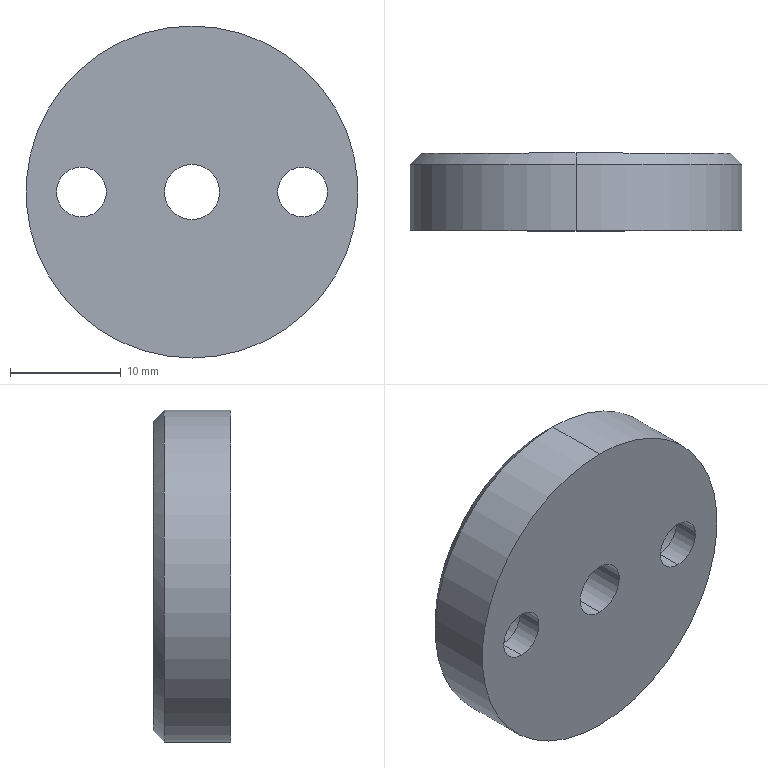Part | STEP file | 手柄盖^回墨刀-350 | 1 solid | 18 faces | box 30 x 7 x 30 mm | volume 4226 mm3 | cylinder 12 | plane 4 | cone 2 | commonest cylinder face diameters 4.5 x4 8 x4 5 x2 30 x2
STEP:
#1=CARTESIAN_POINT('',(-94.996,86.9,-6.23));
#2=VERTEX_POINT('',#1);
#3=CARTESIAN_POINT('',(-94.996,86.9,1.77));
#4=VERTEX_POINT('',#3);
#5=CARTESIAN_POINT('',(-94.996,86.9,-2.23));
#6=DIRECTION('',(0.,1.,0.));
#7=DIRECTION('',(0.,0.,1.));
#8=AXIS2_PLACEMENT_3D('',#5,#6,#7);
#9=CIRCLE('',#8,4.);
#10=EDGE_CURVE('',#2,#4,#9,.T.);
#11=ORIENTED_EDGE('',*,*,#10,.F.);
#12=CARTESIAN_POINT('',(-94.996,91.5,-6.23));
#13=VERTEX_POINT('',#12);
#14=CARTESIAN_POINT('',(-94.996,91.5,-6.23));
#15=DIRECTION('',(0.,1.,0.));
#16=VECTOR('',#15,1000.);
#17=LINE('',#14,#16);
#18=EDGE_CURVE('',#2,#13,#17,.T.);
#19=ORIENTED_EDGE('',*,*,#18,.T.);
#20=CARTESIAN_POINT('',(-94.996,91.5,1.77));
#21=VERTEX_POINT('',#20);
#22=CARTESIAN_POINT('',(-94.996,91.5,-2.23));
#23=DIRECTION('',(0.,1.,0.));
#24=DIRECTION('',(0.,0.,1.));
#25=AXIS2_PLACEMENT_3D('',#22,#23,#24);
#26=CIRCLE('',#25,4.);
#27=EDGE_CURVE('',#13,#21,#26,.T.);
#28=ORIENTED_EDGE('',*,*,#27,.T.);
#29=CARTESIAN_POINT('',(-94.996,91.5,1.77));
#30=DIRECTION('',(0.,1.,0.));
#31=VECTOR('',#30,1000.);
#32=LINE('',#29,#31);
#33=EDGE_CURVE('',#4,#21,#32,.T.);
#34=ORIENTED_EDGE('',*,*,#33,.F.);
#35=EDGE_LOOP('',(#11,#19,#28,#34));
#36=FACE_OUTER_BOUND('',#35,.T.);
#37=CARTESIAN_POINT('',(-94.996,91.5,-2.23));
#38=DIRECTION('',(0.,1.,0.));
#39=DIRECTION('',(0.,0.,1.));
#40=AXIS2_PLACEMENT_3D('',#37,#38,#39);
#41=CYLINDRICAL_SURFACE('',#40,4.);
#42=ADVANCED_FACE('',(#36),#41,.F.);
#43=CARTESIAN_POINT('',(-94.996,84.5,-4.48));
#44=VERTEX_POINT('',#43);
#45=CARTESIAN_POINT('',(-94.996,84.5,0.01978));
#46=VERTEX_POINT('',#45);
#47=CARTESIAN_POINT('',(-94.996,84.5,-2.23));
#48=DIRECTION('',(0.,1.,0.));
#49=DIRECTION('',(0.,0.,1.));
#50=AXIS2_PLACEMENT_3D('',#47,#48,#49);
#51=CIRCLE('',#50,2.25);
#52=EDGE_CURVE('',#44,#46,#51,.T.);
#53=ORIENTED_EDGE('',*,*,#52,.F.);
#54=CARTESIAN_POINT('',(-94.996,86.9,-4.48));
#55=VERTEX_POINT('',#54);
#56=CARTESIAN_POINT('',(-94.996,91.5,-4.48));
#57=DIRECTION('',(0.,1.,0.));
#58=VECTOR('',#57,1000.);
#59=LINE('',#56,#58);
#60=EDGE_CURVE('',#44,#55,#59,.T.);
#61=ORIENTED_EDGE('',*,*,#60,.T.);
#62=CARTESIAN_POINT('',(-94.996,86.9,0.01978));
#63=VERTEX_POINT('',#62);
#64=CARTESIAN_POINT('',(-94.996,86.9,-2.23));
#65=DIRECTION('',(0.,1.,0.));
#66=DIRECTION('',(0.,0.,1.));
#67=AXIS2_PLACEMENT_3D('',#64,#65,#66);
#68=CIRCLE('',#67,2.25);
#69=EDGE_CURVE('',#55,#63,#68,.T.);
#70=ORIENTED_EDGE('',*,*,#69,.T.);
#71=CARTESIAN_POINT('',(-94.996,91.5,0.01978));
#72=DIRECTION('',(0.,1.,0.));
#73=VECTOR('',#72,1000.);
#74=LINE('',#71,#73);
#75=EDGE_CURVE('',#46,#63,#74,.T.);
#76=ORIENTED_EDGE('',*,*,#75,.F.);
#77=EDGE_LOOP('',(#53,#61,#70,#76));
#78=FACE_OUTER_BOUND('',#77,.T.);
#79=CARTESIAN_POINT('',(-94.996,91.5,-2.23));
#80=DIRECTION('',(0.,1.,0.));
#81=DIRECTION('',(0.,0.,1.));
#82=AXIS2_PLACEMENT_3D('',#79,#80,#81);
#83=CYLINDRICAL_SURFACE('',#82,2.25);
#84=ADVANCED_FACE('',(#78),#83,.F.);
#85=CARTESIAN_POINT('',(-114.996,86.9,-6.23));
#86=VERTEX_POINT('',#85);
#87=CARTESIAN_POINT('',(-114.996,86.9,1.77));
#88=VERTEX_POINT('',#87);
#89=CARTESIAN_POINT('',(-114.996,86.9,-2.23));
#90=DIRECTION('',(0.,1.,0.));
#91=DIRECTION('',(0.,0.,1.));
#92=AXIS2_PLACEMENT_3D('',#89,#90,#91);
#93=CIRCLE('',#92,4.);
#94=EDGE_CURVE('',#86,#88,#93,.T.);
#95=ORIENTED_EDGE('',*,*,#94,.F.);
#96=CARTESIAN_POINT('',(-114.996,91.5,-6.23));
#97=VERTEX_POINT('',#96);
#98=CARTESIAN_POINT('',(-114.996,91.5,-6.23));
#99=DIRECTION('',(0.,1.,0.));
#100=VECTOR('',#99,1000.);
#101=LINE('',#98,#100);
#102=EDGE_CURVE('',#86,#97,#101,.T.);
#103=ORIENTED_EDGE('',*,*,#102,.T.);
#104=CARTESIAN_POINT('',(-118.996,91.5,-2.23));
#105=VERTEX_POINT('',#104);
#106=CARTESIAN_POINT('',(-114.996,91.5,-2.23));
#107=DIRECTION('',(0.,1.,0.));
#108=DIRECTION('',(0.,0.,1.));
#109=AXIS2_PLACEMENT_3D('',#106,#107,#108);
#110=CIRCLE('',#109,4.);
#111=EDGE_CURVE('',#97,#105,#110,.T.);
#112=ORIENTED_EDGE('',*,*,#111,.T.);
#113=CARTESIAN_POINT('',(-114.996,91.5,1.77));
#114=VERTEX_POINT('',#113);
#115=CARTESIAN_POINT('',(-114.996,91.5,-2.23));
#116=DIRECTION('',(0.,1.,0.));
#117=DIRECTION('',(0.,0.,1.));
#118=AXIS2_PLACEMENT_3D('',#115,#116,#117);
#119=CIRCLE('',#118,4.);
#120=EDGE_CURVE('',#105,#114,#119,.T.);
#121=ORIENTED_EDGE('',*,*,#120,.T.);
#122=CARTESIAN_POINT('',(-114.996,91.5,1.77));
#123=DIRECTION('',(0.,1.,0.));
#124=VECTOR('',#123,1000.);
#125=LINE('',#122,#124);
#126=EDGE_CURVE('',#88,#114,#125,.T.);
#127=ORIENTED_EDGE('',*,*,#126,.F.);
#128=EDGE_LOOP('',(#95,#103,#112,#121,#127));
#129=FACE_OUTER_BOUND('',#128,.T.);
#130=CARTESIAN_POINT('',(-114.996,91.5,-2.23));
#131=DIRECTION('',(0.,1.,0.));
#132=DIRECTION('',(0.,0.,1.));
#133=AXIS2_PLACEMENT_3D('',#130,#131,#132);
#134=CYLINDRICAL_SURFACE('',#133,4.);
#135=ADVANCED_FACE('',(#129),#134,.F.);
#136=CARTESIAN_POINT('',(-114.996,84.5,-4.48));
#137=VERTEX_POINT('',#136);
#138=CARTESIAN_POINT('',(-114.996,84.5,0.01978));
#139=VERTEX_POINT('',#138);
#140=CARTESIAN_POINT('',(-114.996,84.5,-2.23));
#141=DIRECTION('',(0.,1.,0.));
#142=DIRECTION('',(0.,0.,1.));
#143=AXIS2_PLACEMENT_3D('',#140,#141,#142);
#144=CIRCLE('',#143,2.25);
#145=EDGE_CURVE('',#137,#139,#144,.T.);
#146=ORIENTED_EDGE('',*,*,#145,.F.);
#147=CARTESIAN_POINT('',(-114.996,86.9,-4.48));
#148=VERTEX_POINT('',#147);
#149=CARTESIAN_POINT('',(-114.996,91.5,-4.48));
#150=DIRECTION('',(0.,1.,0.));
#151=VECTOR('',#150,1000.);
#152=LINE('',#149,#151);
#153=EDGE_CURVE('',#137,#148,#152,.T.);
#154=ORIENTED_EDGE('',*,*,#153,.T.);
#155=CARTESIAN_POINT('',(-114.996,86.9,0.01978));
#156=VERTEX_POINT('',#155);
#157=CARTESIAN_POINT('',(-114.996,86.9,-2.23));
#158=DIRECTION('',(0.,1.,0.));
#159=DIRECTION('',(0.,0.,1.));
#160=AXIS2_PLACEMENT_3D('',#157,#158,#159);
#161=CIRCLE('',#160,2.25);
#162=EDGE_CURVE('',#148,#156,#161,.T.);
#163=ORIENTED_EDGE('',*,*,#162,.T.);
#164=CARTESIAN_POINT('',(-114.996,91.5,0.01978));
#165=DIRECTION('',(0.,1.,0.));
#166=VECTOR('',#165,1000.);
#167=LINE('',#164,#166);
#168=EDGE_CURVE('',#139,#156,#167,.T.);
#169=ORIENTED_EDGE('',*,*,#168,.F.);
#170=EDGE_LOOP('',(#146,#154,#163,#169));
#171=FACE_OUTER_BOUND('',#170,.T.);
#172=CARTESIAN_POINT('',(-114.996,91.5,-2.23));
#173=DIRECTION('',(0.,1.,0.));
#174=DIRECTION('',(0.,0.,1.));
#175=AXIS2_PLACEMENT_3D('',#172,#173,#174);
#176=CYLINDRICAL_SURFACE('',#175,2.25);
#177=ADVANCED_FACE('',(#171),#176,.F.);
#178=CARTESIAN_POINT('',(-104.996,84.5,-4.73));
#179=VERTEX_POINT('',#178);
#180=CARTESIAN_POINT('',(-104.996,84.5,0.2698));
#181=VERTEX_POINT('',#180);
#182=CARTESIAN_POINT('',(-104.996,84.5,-2.23));
#183=DIRECTION('',(0.,1.,0.));
#184=DIRECTION('',(0.,0.,1.));
#185=AXIS2_PLACEMENT_3D('',#182,#183,#184);
#186=CIRCLE('',#185,2.5);
#187=EDGE_CURVE('',#179,#181,#186,.T.);
#188=ORIENTED_EDGE('',*,*,#187,.F.);
#189=CARTESIAN_POINT('',(-104.996,91.5,-4.73));
#190=VERTEX_POINT('',#189);
#191=CARTESIAN_POINT('',(-104.996,91.5,-4.73));
#192=DIRECTION('',(0.,1.,0.));
#193=VECTOR('',#192,1000.);
#194=LINE('',#191,#193);
#195=EDGE_CURVE('',#179,#190,#194,.T.);
#196=ORIENTED_EDGE('',*,*,#195,.T.);
#197=CARTESIAN_POINT('',(-104.996,91.5,0.2698));
#198=VERTEX_POINT('',#197);
#199=CARTESIAN_POINT('',(-104.996,91.5,-2.23));
#200=DIRECTION('',(0.,1.,0.));
#201=DIRECTION('',(0.,0.,1.));
#202=AXIS2_PLACEMENT_3D('',#199,#200,#201);
#203=CIRCLE('',#202,2.5);
#204=EDGE_CURVE('',#190,#198,#203,.T.);
#205=ORIENTED_EDGE('',*,*,#204,.T.);
#206=CARTESIAN_POINT('',(-104.996,91.5,0.2698));
#207=DIRECTION('',(0.,1.,0.));
#208=VECTOR('',#207,1000.);
#209=LINE('',#206,#208);
#210=EDGE_CURVE('',#181,#198,#209,.T.);
#211=ORIENTED_EDGE('',*,*,#210,.F.);
#212=EDGE_LOOP('',(#188,#196,#205,#211));
#213=FACE_OUTER_BOUND('',#212,.T.);
#214=CARTESIAN_POINT('',(-104.996,91.5,-2.23));
#215=DIRECTION('',(0.,1.,0.));
#216=DIRECTION('',(0.,0.,1.));
#217=AXIS2_PLACEMENT_3D('',#214,#215,#216);
#218=CYLINDRICAL_SURFACE('',#217,2.5);
#219=ADVANCED_FACE('',(#213),#218,.F.);
#220=CARTESIAN_POINT('',(-104.996,91.5,11.77));
#221=VERTEX_POINT('',#220);
#222=CARTESIAN_POINT('',(-90.996,91.5,-2.23));
#223=VERTEX_POINT('',#222);
#224=CARTESIAN_POINT('',(-104.996,91.5,-2.23));
#225=DIRECTION('',(0.,1.,0.));
#226=DIRECTION('',(0.,0.,1.));
#227=AXIS2_PLACEMENT_3D('',#224,#225,#226);
#228=CIRCLE('',#227,14.);
#229=EDGE_CURVE('',#221,#223,#228,.T.);
#230=ORIENTED_EDGE('',*,*,#229,.F.);
#231=CARTESIAN_POINT('',(-104.996,90.5,12.77));
#232=VERTEX_POINT('',#231);
#233=CARTESIAN_POINT('',(-104.996,91.5,11.77));
#234=DIRECTION('',(0.,-0.7071,0.7071));
#235=VECTOR('',#234,1000.);
#236=LINE('',#233,#235);
#237=EDGE_CURVE('',#221,#232,#236,.T.);
#238=ORIENTED_EDGE('',*,*,#237,.T.);
#239=CARTESIAN_POINT('',(-104.996,90.5,-17.23));
#240=VERTEX_POINT('',#239);
#241=CARTESIAN_POINT('',(-104.996,90.5,-2.23));
#242=DIRECTION('',(0.,-1.,0.));
#243=DIRECTION('',(0.,0.,1.));
#244=AXIS2_PLACEMENT_3D('',#241,#242,#243);
#245=CIRCLE('',#244,15.);
#246=EDGE_CURVE('',#240,#232,#245,.T.);
#247=ORIENTED_EDGE('',*,*,#246,.F.);
#248=CARTESIAN_POINT('',(-104.996,91.5,-16.23));
#249=VERTEX_POINT('',#248);
#250=CARTESIAN_POINT('',(-104.996,91.5,-16.23));
#251=DIRECTION('',(0.,-0.7071,-0.7071));
#252=VECTOR('',#251,1000.);
#253=LINE('',#250,#252);
#254=EDGE_CURVE('',#249,#240,#253,.T.);
#255=ORIENTED_EDGE('',*,*,#254,.F.);
#256=CARTESIAN_POINT('',(-104.996,91.5,-2.23));
#257=DIRECTION('',(0.,1.,0.));
#258=DIRECTION('',(0.,0.,1.));
#259=AXIS2_PLACEMENT_3D('',#256,#257,#258);
#260=CIRCLE('',#259,14.);
#261=EDGE_CURVE('',#223,#249,#260,.T.);
#262=ORIENTED_EDGE('',*,*,#261,.F.);
#263=EDGE_LOOP('',(#230,#238,#247,#255,#262));
#264=FACE_OUTER_BOUND('',#263,.T.);
#265=CARTESIAN_POINT('',(-104.996,91.5,-2.23));
#266=DIRECTION('',(0.,-1.,0.));
#267=DIRECTION('',(0.,0.,-1.));
#268=AXIS2_PLACEMENT_3D('',#265,#266,#267);
#269=CONICAL_SURFACE('',#268,14.,0.7854);
#270=ADVANCED_FACE('',(#264),#269,.T.);
#271=ORIENTED_EDGE('',*,*,#246,.T.);
#272=CARTESIAN_POINT('',(-104.996,84.5,12.77));
#273=VERTEX_POINT('',#272);
#274=CARTESIAN_POINT('',(-104.996,91.5,12.77));
#275=DIRECTION('',(0.,-1.,0.));
#276=VECTOR('',#275,1000.);
#277=LINE('',#274,#276);
#278=EDGE_CURVE('',#232,#273,#277,.T.);
#279=ORIENTED_EDGE('',*,*,#278,.T.);
#280=CARTESIAN_POINT('',(-104.996,84.5,-17.23));
#281=VERTEX_POINT('',#280);
#282=CARTESIAN_POINT('',(-104.996,84.5,-2.23));
#283=DIRECTION('',(0.,1.,0.));
#284=DIRECTION('',(0.,0.,1.));
#285=AXIS2_PLACEMENT_3D('',#282,#283,#284);
#286=CIRCLE('',#285,15.);
#287=EDGE_CURVE('',#273,#281,#286,.T.);
#288=ORIENTED_EDGE('',*,*,#287,.T.);
#289=CARTESIAN_POINT('',(-104.996,91.5,-17.23));
#290=DIRECTION('',(0.,-1.,0.));
#291=VECTOR('',#290,1000.);
#292=LINE('',#289,#291);
#293=EDGE_CURVE('',#240,#281,#292,.T.);
#294=ORIENTED_EDGE('',*,*,#293,.F.);
#295=EDGE_LOOP('',(#271,#279,#288,#294));
#296=FACE_OUTER_BOUND('',#295,.T.);
#297=CARTESIAN_POINT('',(-104.996,91.5,-2.23));
#298=DIRECTION('',(0.,-1.,0.));
#299=DIRECTION('',(0.,0.,-1.));
#300=AXIS2_PLACEMENT_3D('',#297,#298,#299);
#301=CYLINDRICAL_SURFACE('',#300,15.);
#302=ADVANCED_FACE('',(#296),#301,.T.);
#303=ORIENTED_EDGE('',*,*,#278,.F.);
#304=CARTESIAN_POINT('',(-104.996,90.5,-2.23));
#305=DIRECTION('',(0.,-1.,0.));
#306=DIRECTION('',(0.,0.,1.));
#307=AXIS2_PLACEMENT_3D('',#304,#305,#306);
#308=CIRCLE('',#307,15.);
#309=EDGE_CURVE('',#232,#240,#308,.T.);
#310=ORIENTED_EDGE('',*,*,#309,.T.);
#311=ORIENTED_EDGE('',*,*,#293,.T.);
#312=CARTESIAN_POINT('',(-104.996,84.5,-2.23));
#313=DIRECTION('',(0.,1.,0.));
#314=DIRECTION('',(0.,0.,1.));
#315=AXIS2_PLACEMENT_3D('',#312,#313,#314);
#316=CIRCLE('',#315,15.);
#317=EDGE_CURVE('',#281,#273,#316,.T.);
#318=ORIENTED_EDGE('',*,*,#317,.T.);
#319=EDGE_LOOP('',(#303,#310,#311,#318));
#320=FACE_OUTER_BOUND('',#319,.T.);
#321=CARTESIAN_POINT('',(-104.996,91.5,-2.23));
#322=DIRECTION('',(0.,-1.,0.));
#323=DIRECTION('',(0.,0.,-1.));
#324=AXIS2_PLACEMENT_3D('',#321,#322,#323);
#325=CYLINDRICAL_SURFACE('',#324,15.);
#326=ADVANCED_FACE('',(#320),#325,.T.);
#327=CARTESIAN_POINT('',(-104.996,91.5,-2.23));
#328=DIRECTION('',(0.,1.,0.));
#329=DIRECTION('',(0.,0.,1.));
#330=AXIS2_PLACEMENT_3D('',#327,#328,#329);
#331=CIRCLE('',#330,2.5);
#332=EDGE_CURVE('',#198,#190,#331,.T.);
#333=ORIENTED_EDGE('',*,*,#332,.F.);
#334=ORIENTED_EDGE('',*,*,#204,.F.);
#335=EDGE_LOOP('',(#333,#334));
#336=FACE_BOUND('',#335,.T.);
#337=CARTESIAN_POINT('',(-104.996,91.5,-2.23));
#338=DIRECTION('',(0.,1.,0.));
#339=DIRECTION('',(0.,0.,1.));
#340=AXIS2_PLACEMENT_3D('',#337,#338,#339);
#341=CIRCLE('',#340,14.);
#342=EDGE_CURVE('',#105,#221,#341,.T.);
#343=ORIENTED_EDGE('',*,*,#342,.T.);
#344=ORIENTED_EDGE('',*,*,#229,.T.);
#345=CARTESIAN_POINT('',(-94.996,91.5,-2.23));
#346=DIRECTION('',(0.,1.,0.));
#347=DIRECTION('',(0.,0.,1.));
#348=AXIS2_PLACEMENT_3D('',#345,#346,#347);
#349=CIRCLE('',#348,4.);
#350=EDGE_CURVE('',#21,#223,#349,.T.);
#351=ORIENTED_EDGE('',*,*,#350,.F.);
#352=ORIENTED_EDGE('',*,*,#27,.F.);
#353=CARTESIAN_POINT('',(-94.996,91.5,-2.23));
#354=DIRECTION('',(0.,1.,0.));
#355=DIRECTION('',(0.,0.,1.));
#356=AXIS2_PLACEMENT_3D('',#353,#354,#355);
#357=CIRCLE('',#356,4.);
#358=EDGE_CURVE('',#223,#13,#357,.T.);
#359=ORIENTED_EDGE('',*,*,#358,.F.);
#360=ORIENTED_EDGE('',*,*,#261,.T.);
#361=CARTESIAN_POINT('',(-104.996,91.5,-2.23));
#362=DIRECTION('',(0.,1.,0.));
#363=DIRECTION('',(0.,0.,1.));
#364=AXIS2_PLACEMENT_3D('',#361,#362,#363);
#365=CIRCLE('',#364,14.);
#366=EDGE_CURVE('',#249,#105,#365,.T.);
#367=ORIENTED_EDGE('',*,*,#366,.T.);
#368=ORIENTED_EDGE('',*,*,#111,.F.);
#369=CARTESIAN_POINT('',(-114.996,91.5,-2.23));
#370=DIRECTION('',(0.,1.,0.));
#371=DIRECTION('',(0.,0.,1.));
#372=AXIS2_PLACEMENT_3D('',#369,#370,#371);
#373=CIRCLE('',#372,4.);
#374=EDGE_CURVE('',#114,#97,#373,.T.);
#375=ORIENTED_EDGE('',*,*,#374,.F.);
#376=ORIENTED_EDGE('',*,*,#120,.F.);
#377=EDGE_LOOP('',(#343,#344,#351,#352,#359,#360,#367,#368,#375,#376));
#378=FACE_OUTER_BOUND('',#377,.T.);
#379=CARTESIAN_POINT('',(-104.996,91.5,-2.23));
#380=DIRECTION('',(0.,1.,0.));
#381=DIRECTION('',(0.,0.,1.));
#382=AXIS2_PLACEMENT_3D('',#379,#380,#381);
#383=PLANE('',#382);
#384=ADVANCED_FACE('',(#336,#378),#383,.T.);
#385=CARTESIAN_POINT('',(-94.996,84.5,-2.23));
#386=DIRECTION('',(0.,1.,0.));
#387=DIRECTION('',(0.,0.,1.));
#388=AXIS2_PLACEMENT_3D('',#385,#386,#387);
#389=CIRCLE('',#388,2.25);
#390=EDGE_CURVE('',#46,#44,#389,.T.);
#391=ORIENTED_EDGE('',*,*,#390,.T.);
#392=ORIENTED_EDGE('',*,*,#52,.T.);
#393=EDGE_LOOP('',(#391,#392));
#394=FACE_BOUND('',#393,.T.);
#395=CARTESIAN_POINT('',(-114.996,84.5,-2.23));
#396=DIRECTION('',(0.,1.,0.));
#397=DIRECTION('',(0.,0.,1.));
#398=AXIS2_PLACEMENT_3D('',#395,#396,#397);
#399=CIRCLE('',#398,2.25);
#400=EDGE_CURVE('',#139,#137,#399,.T.);
#401=ORIENTED_EDGE('',*,*,#400,.T.);
#402=ORIENTED_EDGE('',*,*,#145,.T.);
#403=EDGE_LOOP('',(#401,#402));
#404=FACE_BOUND('',#403,.T.);
#405=CARTESIAN_POINT('',(-104.996,84.5,-2.23));
#406=DIRECTION('',(0.,1.,0.));
#407=DIRECTION('',(0.,0.,1.));
#408=AXIS2_PLACEMENT_3D('',#405,#406,#407);
#409=CIRCLE('',#408,2.5);
#410=EDGE_CURVE('',#181,#179,#409,.T.);
#411=ORIENTED_EDGE('',*,*,#410,.T.);
#412=ORIENTED_EDGE('',*,*,#187,.T.);
#413=EDGE_LOOP('',(#411,#412));
#414=FACE_BOUND('',#413,.T.);
#415=ORIENTED_EDGE('',*,*,#317,.F.);
#416=ORIENTED_EDGE('',*,*,#287,.F.);
#417=EDGE_LOOP('',(#415,#416));
#418=FACE_OUTER_BOUND('',#417,.T.);
#419=CARTESIAN_POINT('',(-104.996,84.5,-2.23));
#420=DIRECTION('',(0.,1.,0.));
#421=DIRECTION('',(0.,0.,1.));
#422=AXIS2_PLACEMENT_3D('',#419,#420,#421);
#423=PLANE('',#422);
#424=ADVANCED_FACE('',(#394,#404,#414,#418),#423,.F.);
#425=ORIENTED_EDGE('',*,*,#237,.F.);
#426=ORIENTED_EDGE('',*,*,#342,.F.);
#427=ORIENTED_EDGE('',*,*,#366,.F.);
#428=ORIENTED_EDGE('',*,*,#254,.T.);
#429=ORIENTED_EDGE('',*,*,#309,.F.);
#430=EDGE_LOOP('',(#425,#426,#427,#428,#429));
#431=FACE_OUTER_BOUND('',#430,.T.);
#432=CARTESIAN_POINT('',(-104.996,91.5,-2.23));
#433=DIRECTION('',(0.,-1.,0.));
#434=DIRECTION('',(0.,0.,-1.));
#435=AXIS2_PLACEMENT_3D('',#432,#433,#434);
#436=CONICAL_SURFACE('',#435,14.,0.7854);
#437=ADVANCED_FACE('',(#431),#436,.T.);
#438=ORIENTED_EDGE('',*,*,#195,.F.);
#439=ORIENTED_EDGE('',*,*,#410,.F.);
#440=ORIENTED_EDGE('',*,*,#210,.T.);
#441=ORIENTED_EDGE('',*,*,#332,.T.);
#442=EDGE_LOOP('',(#438,#439,#440,#441));
#443=FACE_OUTER_BOUND('',#442,.T.);
#444=CARTESIAN_POINT('',(-104.996,91.5,-2.23));
#445=DIRECTION('',(0.,1.,0.));
#446=DIRECTION('',(0.,0.,1.));
#447=AXIS2_PLACEMENT_3D('',#444,#445,#446);
#448=CYLINDRICAL_SURFACE('',#447,2.5);
#449=ADVANCED_FACE('',(#443),#448,.F.);
#450=ORIENTED_EDGE('',*,*,#153,.F.);
#451=ORIENTED_EDGE('',*,*,#400,.F.);
#452=ORIENTED_EDGE('',*,*,#168,.T.);
#453=CARTESIAN_POINT('',(-114.996,86.9,-2.23));
#454=DIRECTION('',(0.,1.,0.));
#455=DIRECTION('',(0.,0.,1.));
#456=AXIS2_PLACEMENT_3D('',#453,#454,#455);
#457=CIRCLE('',#456,2.25);
#458=EDGE_CURVE('',#156,#148,#457,.T.);
#459=ORIENTED_EDGE('',*,*,#458,.T.);
#460=EDGE_LOOP('',(#450,#451,#452,#459));
#461=FACE_OUTER_BOUND('',#460,.T.);
#462=CARTESIAN_POINT('',(-114.996,91.5,-2.23));
#463=DIRECTION('',(0.,1.,0.));
#464=DIRECTION('',(0.,0.,1.));
#465=AXIS2_PLACEMENT_3D('',#462,#463,#464);
#466=CYLINDRICAL_SURFACE('',#465,2.25);
#467=ADVANCED_FACE('',(#461),#466,.F.);
#468=ORIENTED_EDGE('',*,*,#458,.F.);
#469=ORIENTED_EDGE('',*,*,#162,.F.);
#470=EDGE_LOOP('',(#468,#469));
#471=FACE_BOUND('',#470,.T.);
#472=CARTESIAN_POINT('',(-114.996,86.9,-2.23));
#473=DIRECTION('',(0.,1.,0.));
#474=DIRECTION('',(0.,0.,1.));
#475=AXIS2_PLACEMENT_3D('',#472,#473,#474);
#476=CIRCLE('',#475,4.);
#477=EDGE_CURVE('',#88,#86,#476,.T.);
#478=ORIENTED_EDGE('',*,*,#477,.T.);
#479=ORIENTED_EDGE('',*,*,#94,.T.);
#480=EDGE_LOOP('',(#478,#479));
#481=FACE_OUTER_BOUND('',#480,.T.);
#482=CARTESIAN_POINT('',(-112.746,86.9,-2.23));
#483=DIRECTION('',(0.,-1.,0.));
#484=DIRECTION('',(0.,0.,-1.));
#485=AXIS2_PLACEMENT_3D('',#482,#483,#484);
#486=PLANE('',#485);
#487=ADVANCED_FACE('',(#471,#481),#486,.F.);
#488=ORIENTED_EDGE('',*,*,#102,.F.);
#489=ORIENTED_EDGE('',*,*,#477,.F.);
#490=ORIENTED_EDGE('',*,*,#126,.T.);
#491=ORIENTED_EDGE('',*,*,#374,.T.);
#492=EDGE_LOOP('',(#488,#489,#490,#491));
#493=FACE_OUTER_BOUND('',#492,.T.);
#494=CARTESIAN_POINT('',(-114.996,91.5,-2.23));
#495=DIRECTION('',(0.,1.,0.));
#496=DIRECTION('',(0.,0.,1.));
#497=AXIS2_PLACEMENT_3D('',#494,#495,#496);
#498=CYLINDRICAL_SURFACE('',#497,4.);
#499=ADVANCED_FACE('',(#493),#498,.F.);
#500=ORIENTED_EDGE('',*,*,#60,.F.);
#501=ORIENTED_EDGE('',*,*,#390,.F.);
#502=ORIENTED_EDGE('',*,*,#75,.T.);
#503=CARTESIAN_POINT('',(-94.996,86.9,-2.23));
#504=DIRECTION('',(0.,1.,0.));
#505=DIRECTION('',(0.,0.,1.));
#506=AXIS2_PLACEMENT_3D('',#503,#504,#505);
#507=CIRCLE('',#506,2.25);
#508=EDGE_CURVE('',#63,#55,#507,.T.);
#509=ORIENTED_EDGE('',*,*,#508,.T.);
#510=EDGE_LOOP('',(#500,#501,#502,#509));
#511=FACE_OUTER_BOUND('',#510,.T.);
#512=CARTESIAN_POINT('',(-94.996,91.5,-2.23));
#513=DIRECTION('',(0.,1.,0.));
#514=DIRECTION('',(0.,0.,1.));
#515=AXIS2_PLACEMENT_3D('',#512,#513,#514);
#516=CYLINDRICAL_SURFACE('',#515,2.25);
#517=ADVANCED_FACE('',(#511),#516,.F.);
#518=ORIENTED_EDGE('',*,*,#508,.F.);
#519=ORIENTED_EDGE('',*,*,#69,.F.);
#520=EDGE_LOOP('',(#518,#519));
#521=FACE_BOUND('',#520,.T.);
#522=CARTESIAN_POINT('',(-94.996,86.9,-2.23));
#523=DIRECTION('',(0.,1.,0.));
#524=DIRECTION('',(0.,0.,1.));
#525=AXIS2_PLACEMENT_3D('',#522,#523,#524);
#526=CIRCLE('',#525,4.);
#527=EDGE_CURVE('',#4,#2,#526,.T.);
#528=ORIENTED_EDGE('',*,*,#527,.T.);
#529=ORIENTED_EDGE('',*,*,#10,.T.);
#530=EDGE_LOOP('',(#528,#529));
#531=FACE_OUTER_BOUND('',#530,.T.);
#532=CARTESIAN_POINT('',(-92.746,86.9,-2.23));
#533=DIRECTION('',(0.,-1.,0.));
#534=DIRECTION('',(0.,0.,-1.));
#535=AXIS2_PLACEMENT_3D('',#532,#533,#534);
#536=PLANE('',#535);
#537=ADVANCED_FACE('',(#521,#531),#536,.F.);
#538=ORIENTED_EDGE('',*,*,#18,.F.);
#539=ORIENTED_EDGE('',*,*,#527,.F.);
#540=ORIENTED_EDGE('',*,*,#33,.T.);
#541=ORIENTED_EDGE('',*,*,#350,.T.);
#542=ORIENTED_EDGE('',*,*,#358,.T.);
#543=EDGE_LOOP('',(#538,#539,#540,#541,#542));
#544=FACE_OUTER_BOUND('',#543,.T.);
#545=CARTESIAN_POINT('',(-94.996,91.5,-2.23));
#546=DIRECTION('',(0.,1.,0.));
#547=DIRECTION('',(0.,0.,1.));
#548=AXIS2_PLACEMENT_3D('',#545,#546,#547);
#549=CYLINDRICAL_SURFACE('',#548,4.);
#550=ADVANCED_FACE('',(#544),#549,.F.);
#551=CLOSED_SHELL('',(#42,#84,#135,#177,#219,#270,#302,#326,#384,#424,#437,#449,#467,#487,#499,#517,#537,#550));
#552=MANIFOLD_SOLID_BREP('',#551);
#553=CARTESIAN_POINT('',(0.,0.,0.));
#554=DIRECTION('',(0.,0.,1.));
#555=DIRECTION('',(1.,0.,0.));
#556=AXIS2_PLACEMENT_3D('',#553,#554,#555);
#557=(LENGTH_UNIT()NAMED_UNIT(*)SI_UNIT(.MILLI.,.METRE.));
#558=UNCERTAINTY_MEASURE_WITH_UNIT(LENGTH_MEASURE(0.00001),#557,'','');
#559=(NAMED_UNIT(*)PLANE_ANGLE_UNIT()SI_UNIT($,.RADIAN.));
#560=(NAMED_UNIT(*)SI_UNIT($,.STERADIAN.)SOLID_ANGLE_UNIT());
#561=(GEOMETRIC_REPRESENTATION_CONTEXT(3)GLOBAL_UNCERTAINTY_ASSIGNED_CONTEXT((#558))GLOBAL_UNIT_ASSIGNED_CONTEXT((#557,#559,#560))REPRESENTATION_CONTEXT('',''));
#562=ADVANCED_BREP_SHAPE_REPRESENTATION('',(#552,#556),#561);